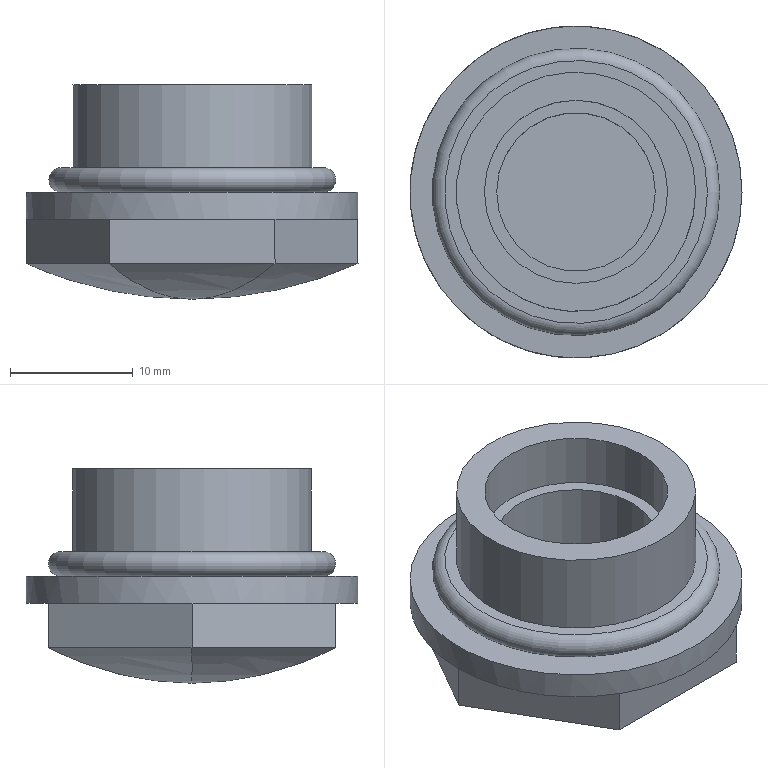Part | NX | features DATUM_CSYS 8, SKETCH 7, EXTRUDE 6, EXTRACT_BODY 5, EXTRACT_STRING 5, BLEND 2, Pattern Geometry 2, UNITE 2, FILL_HOLE 1, SYMBOLIC_THREAD 1, THICKEN_SHEET 1 | 1 solid | 35 faces | box 27 x 27 x 17.442 mm | volume 4366 mm3 | plane 18 | spline 12 | cylinder 4 | torus 1 | commonest cylinder face diameters 12.9 x1 14.9 x1 19.46 x1 27 x1